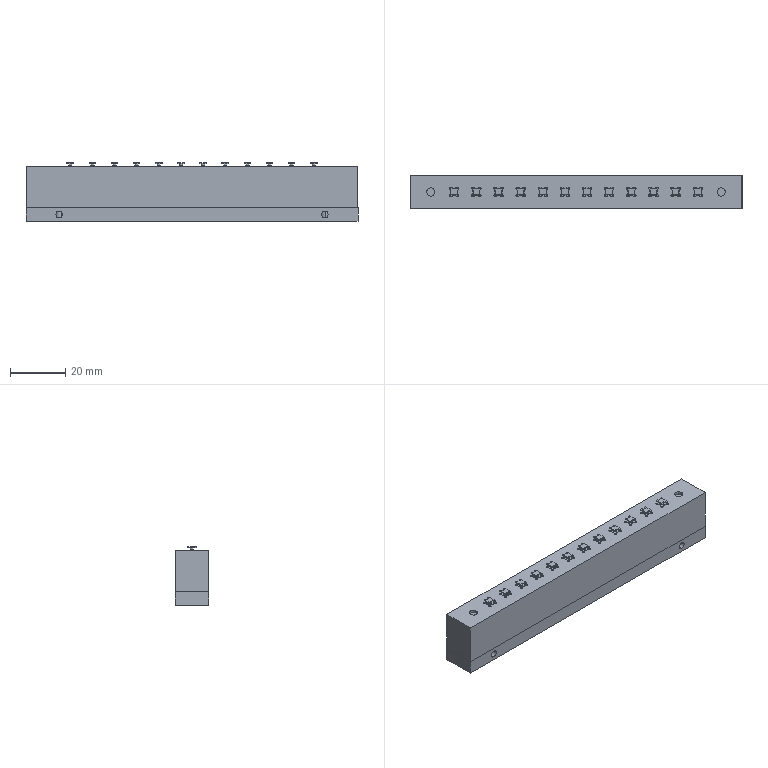Part | SolidWorks | 33 solids | 1120 faces | box 120 x 12 x 21.25 mm | volume 21373 mm3 | plane 621 | cylinder 271 | cone 172 | spline 56 | commonest cylinder face diameters 0.8 x72 2 x54 0.1 x48 1 x24 1.2 x24 3 x16